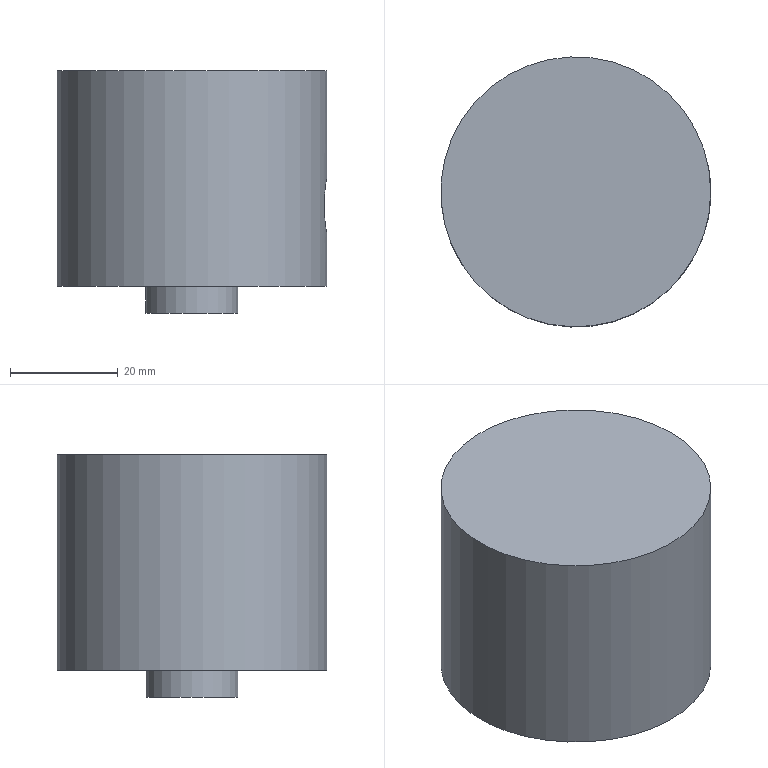Part | NX | features solid 2 | 1 solid | 9 faces | box 50 x 50 x 45 mm | volume 78899 mm3 | plane 5 | cylinder 4 | commonest cylinder face diameters 6 x1 10 x1 17 x1 50 x1
STEP:
#1=CARTESIAN_POINT('',(-1115.,285.,60.));
#2=VERTEX_POINT('',#1);
#3=CARTESIAN_POINT('',(-1140.,285.,60.));
#4=DIRECTION('',(0.,0.,1.));
#5=DIRECTION('',(1.,0.,0.));
#6=AXIS2_PLACEMENT_3D('',#3,#4,#5);
#7=CIRCLE('',#6,25.);
#8=EDGE_CURVE('',#2,#2,#7,.F.);
#9=ORIENTED_EDGE('',*,*,#8,.F.);
#10=EDGE_LOOP('',(#9));
#11=FACE_BOUND('',#10,.T.);
#12=CARTESIAN_POINT('',(-1140.,285.,60.));
#13=DIRECTION('',(0.,0.,1.));
#14=DIRECTION('',(1.,0.,0.));
#15=AXIS2_PLACEMENT_3D('',#12,#13,#14);
#16=PLANE('',#15);
#17=ADVANCED_FACE('',(#11),#16,.T.);
#18=ORIENTED_EDGE('',*,*,#8,.T.);
#19=EDGE_LOOP('',(#18));
#20=FACE_BOUND('',#19,.T.);
#21=CARTESIAN_POINT('',(-1115.004,284.534,39.978));
#22=VERTEX_POINT('',#21);
#23=CARTESIAN_POINT('',(-1115.321,280.732,38.535));
#24=CARTESIAN_POINT('',(-1114.881,284.483,40.518));
#25=CARTESIAN_POINT('',(-1115.18,288.54,39.261));
#26=CARTESIAN_POINT('',(-1115.626,290.516,35.523));
#27=CARTESIAN_POINT('',(-1115.32,289.265,31.461));
#28=CARTESIAN_POINT('',(-1114.882,285.52,29.485));
#29=CARTESIAN_POINT('',(-1115.179,281.466,30.732));
#30=CARTESIAN_POINT('',(-1115.626,279.484,34.479));
#31=CARTESIAN_POINT('',(-1115.321,280.732,38.535));
#32=CARTESIAN_POINT('',(-1114.881,284.483,40.518));
#33=CARTESIAN_POINT('',(-1115.18,288.54,39.261));
#34=B_SPLINE_CURVE_WITH_KNOTS('',3,(#23,#24,#25,#26,#27,#28,#29,#30,#31,#32,#33),.UNSPECIFIED.,.T.,.F.,(1,1,1,1,1,1,1,1,1,1,1,1,1,1,1),(-0.01175,-0.007835,-0.003918,0.,0.003918,0.007835,0.01175,0.01567,0.01959,0.02351,0.02742,0.03134,0.03526,0.03918,0.04309),.UNSPECIFIED.);
#35=EDGE_CURVE('',#22,#22,#34,.T.);
#36=ORIENTED_EDGE('',*,*,#35,.T.);
#37=EDGE_LOOP('',(#36));
#38=FACE_BOUND('',#37,.T.);
#39=CARTESIAN_POINT('',(-1115.,285.,20.));
#40=VERTEX_POINT('',#39);
#41=CARTESIAN_POINT('',(-1140.,285.,20.));
#42=DIRECTION('',(0.,0.,1.));
#43=DIRECTION('',(1.,0.,0.));
#44=AXIS2_PLACEMENT_3D('',#41,#42,#43);
#45=CIRCLE('',#44,25.);
#46=EDGE_CURVE('',#40,#40,#45,.T.);
#47=ORIENTED_EDGE('',*,*,#46,.T.);
#48=EDGE_LOOP('',(#47));
#49=FACE_BOUND('',#48,.T.);
#50=CARTESIAN_POINT('',(-1140.,285.,50.));
#51=DIRECTION('',(0.,0.,-1.));
#52=DIRECTION('',(-1.,0.,0.));
#53=AXIS2_PLACEMENT_3D('',#50,#51,#52);
#54=CYLINDRICAL_SURFACE('',#53,25.);
#55=ADVANCED_FACE('',(#20,#38,#49),#54,.T.);
#56=CARTESIAN_POINT('',(-1131.5,285.,20.));
#57=VERTEX_POINT('',#56);
#58=CARTESIAN_POINT('',(-1140.,285.,20.));
#59=DIRECTION('',(0.,0.,1.));
#60=DIRECTION('',(1.,0.,0.));
#61=AXIS2_PLACEMENT_3D('',#58,#59,#60);
#62=CIRCLE('',#61,8.5);
#63=EDGE_CURVE('',#57,#57,#62,.T.);
#64=ORIENTED_EDGE('',*,*,#63,.T.);
#65=EDGE_LOOP('',(#64));
#66=FACE_BOUND('',#65,.T.);
#67=ORIENTED_EDGE('',*,*,#46,.F.);
#68=EDGE_LOOP('',(#67));
#69=FACE_BOUND('',#68,.T.);
#70=CARTESIAN_POINT('',(-1140.,285.,20.));
#71=DIRECTION('',(0.,0.,1.));
#72=DIRECTION('',(1.,0.,0.));
#73=AXIS2_PLACEMENT_3D('',#70,#71,#72);
#74=PLANE('',#73);
#75=ADVANCED_FACE('',(#66,#69),#74,.F.);
#76=CARTESIAN_POINT('',(-1131.5,285.,15.));
#77=VERTEX_POINT('',#76);
#78=CARTESIAN_POINT('',(-1140.,285.,15.));
#79=DIRECTION('',(0.,0.,1.));
#80=DIRECTION('',(1.,0.,0.));
#81=AXIS2_PLACEMENT_3D('',#78,#79,#80);
#82=CIRCLE('',#81,8.5);
#83=EDGE_CURVE('',#77,#77,#82,.T.);
#84=ORIENTED_EDGE('',*,*,#83,.T.);
#85=EDGE_LOOP('',(#84));
#86=FACE_BOUND('',#85,.T.);
#87=ORIENTED_EDGE('',*,*,#63,.F.);
#88=EDGE_LOOP('',(#87));
#89=FACE_BOUND('',#88,.T.);
#90=CARTESIAN_POINT('',(-1140.,285.,15.));
#91=DIRECTION('',(0.,0.,1.));
#92=DIRECTION('',(1.,0.,0.));
#93=AXIS2_PLACEMENT_3D('',#90,#91,#92);
#94=CYLINDRICAL_SURFACE('',#93,8.5);
#95=ADVANCED_FACE('',(#86,#89),#94,.T.);
#96=ORIENTED_EDGE('',*,*,#83,.F.);
#97=EDGE_LOOP('',(#96));
#98=FACE_BOUND('',#97,.T.);
#99=CARTESIAN_POINT('',(-1140.,285.,15.));
#100=DIRECTION('',(0.,0.,1.));
#101=DIRECTION('',(1.,0.,0.));
#102=AXIS2_PLACEMENT_3D('',#99,#100,#101);
#103=PLANE('',#102);
#104=ADVANCED_FACE('',(#98),#103,.F.);
#105=CARTESIAN_POINT('',(-1116.,285.,30.));
#106=VERTEX_POINT('',#105);
#107=CARTESIAN_POINT('',(-1116.,285.,35.));
#108=DIRECTION('',(1.,0.,0.));
#109=DIRECTION('',(0.,0.,-1.));
#110=AXIS2_PLACEMENT_3D('',#107,#108,#109);
#111=CIRCLE('',#110,5.);
#112=EDGE_CURVE('',#106,#106,#111,.T.);
#113=ORIENTED_EDGE('',*,*,#112,.F.);
#114=EDGE_LOOP('',(#113));
#115=FACE_BOUND('',#114,.T.);
#116=ORIENTED_EDGE('',*,*,#35,.F.);
#117=EDGE_LOOP('',(#116));
#118=FACE_BOUND('',#117,.T.);
#119=CARTESIAN_POINT('',(-1109.5,285.,35.));
#120=DIRECTION('',(1.,0.,0.));
#121=DIRECTION('',(0.,0.,-1.));
#122=AXIS2_PLACEMENT_3D('',#119,#120,#121);
#123=CYLINDRICAL_SURFACE('',#122,5.);
#124=ADVANCED_FACE('',(#115,#118),#123,.F.);
#125=CARTESIAN_POINT('',(-1116.,285.,32.));
#126=VERTEX_POINT('',#125);
#127=CARTESIAN_POINT('',(-1116.,285.,35.));
#128=DIRECTION('',(1.,0.,0.));
#129=DIRECTION('',(0.,0.,-1.));
#130=AXIS2_PLACEMENT_3D('',#127,#128,#129);
#131=CIRCLE('',#130,3.);
#132=EDGE_CURVE('',#126,#126,#131,.F.);
#133=ORIENTED_EDGE('',*,*,#132,.T.);
#134=EDGE_LOOP('',(#133));
#135=FACE_BOUND('',#134,.T.);
#136=ORIENTED_EDGE('',*,*,#112,.T.);
#137=EDGE_LOOP('',(#136));
#138=FACE_BOUND('',#137,.T.);
#139=CARTESIAN_POINT('',(-1116.,285.,35.));
#140=DIRECTION('',(1.,0.,0.));
#141=DIRECTION('',(0.,0.,-1.));
#142=AXIS2_PLACEMENT_3D('',#139,#140,#141);
#143=PLANE('',#142);
#144=ADVANCED_FACE('',(#135,#138),#143,.T.);
#145=CARTESIAN_POINT('',(-1141.,285.,38.));
#146=VERTEX_POINT('',#145);
#147=CARTESIAN_POINT('',(-1141.,285.,35.));
#148=DIRECTION('',(-1.,0.,0.));
#149=DIRECTION('',(0.,0.,1.));
#150=AXIS2_PLACEMENT_3D('',#147,#148,#149);
#151=CIRCLE('',#150,3.);
#152=EDGE_CURVE('',#146,#146,#151,.T.);
#153=ORIENTED_EDGE('',*,*,#152,.F.);
#154=EDGE_LOOP('',(#153));
#155=FACE_BOUND('',#154,.T.);
#156=CARTESIAN_POINT('',(-1141.,285.,35.));
#157=DIRECTION('',(-1.,0.,0.));
#158=DIRECTION('',(0.,0.,1.));
#159=AXIS2_PLACEMENT_3D('',#156,#157,#158);
#160=PLANE('',#159);
#161=ADVANCED_FACE('',(#155),#160,.F.);
#162=ORIENTED_EDGE('',*,*,#152,.T.);
#163=EDGE_LOOP('',(#162));
#164=FACE_BOUND('',#163,.T.);
#165=ORIENTED_EDGE('',*,*,#132,.F.);
#166=EDGE_LOOP('',(#165));
#167=FACE_BOUND('',#166,.T.);
#168=CARTESIAN_POINT('',(-1109.5,285.,35.));
#169=DIRECTION('',(-1.,0.,0.));
#170=DIRECTION('',(0.,0.,1.));
#171=AXIS2_PLACEMENT_3D('',#168,#169,#170);
#172=CYLINDRICAL_SURFACE('',#171,3.);
#173=ADVANCED_FACE('',(#164,#167),#172,.F.);
#174=CLOSED_SHELL('',(#17,#55,#75,#95,#104,#124,#144,#161,#173));
#175=MANIFOLD_SOLID_BREP('',#174);
#176=(LENGTH_UNIT()NAMED_UNIT(*)SI_UNIT(.MILLI.,.METRE.));
#177=UNCERTAINTY_MEASURE_WITH_UNIT(LENGTH_MEASURE(0.0508),#176,'','');
#178=(NAMED_UNIT(*)PLANE_ANGLE_UNIT()SI_UNIT($,.RADIAN.));
#179=(NAMED_UNIT(*)SI_UNIT($,.STERADIAN.)SOLID_ANGLE_UNIT());
#180=(GEOMETRIC_REPRESENTATION_CONTEXT(3)GLOBAL_UNCERTAINTY_ASSIGNED_CONTEXT((#177))GLOBAL_UNIT_ASSIGNED_CONTEXT((#176,#178,#179))REPRESENTATION_CONTEXT('',''));
#181=ADVANCED_BREP_SHAPE_REPRESENTATION('',(#175),#180);